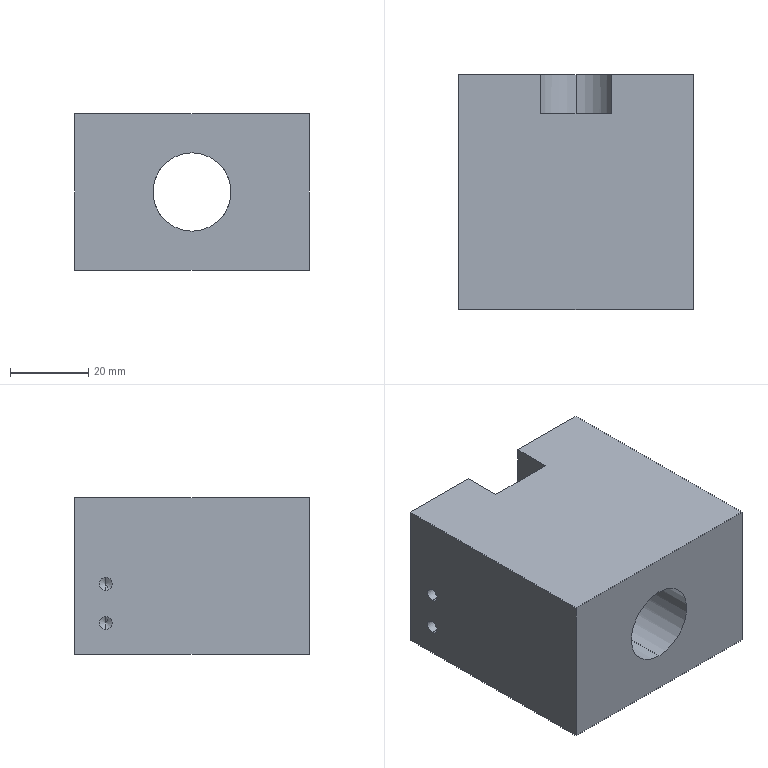Part | STEP file | PN_0053 | 1 solid | 43 faces | box 60 x 60 x 40 mm | volume 121912 mm3 | cylinder 18 | cone 16 | plane 9 | commonest cylinder face diameters 4.2 x8 3.3 x4 4 x4 20 x2